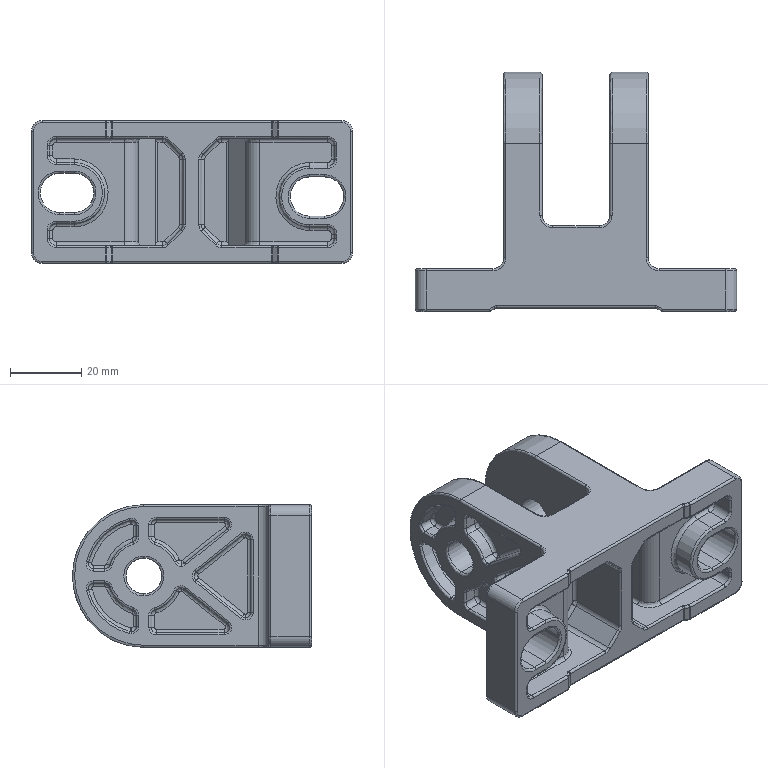Part | SolidWorks | features BaseBody 1 | 1 solid | 525 faces | box 90 x 67 x 40 mm | volume 62935 mm3 | cylinder 239 | spline 190 | plane 84 | torus 12 | commonest cylinder face diameters 1.2 x92 2 x54 3 x43 4 x16 6 x8 20 x8